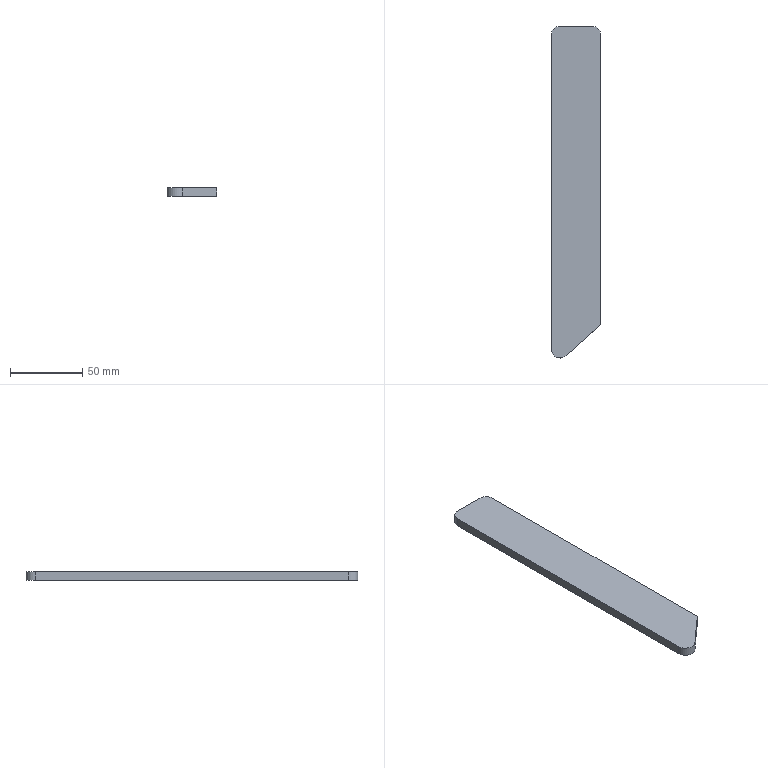Part | SolidWorks | features FlatPattern 1, SMBaseFlange 1, SheetMetal 1 | 1 solid | 9 faces | box 34.572 x 229.825 x 6 mm | volume 45739 mm3 | plane 6 | cylinder 3 | commonest cylinder face diameters 13 x3
STEP:
#1=CARTESIAN_POINT('',(34.572,168.202,0.));
#2=VERTEX_POINT('',#1);
#3=CARTESIAN_POINT('',(34.572,368.497,0.));
#4=VERTEX_POINT('',#3);
#5=CARTESIAN_POINT('',(34.572,168.202,0.));
#6=DIRECTION('',(0.,1.,0.));
#7=VECTOR('',#6,1000.);
#8=LINE('',#5,#7);
#9=EDGE_CURVE('',#2,#4,#8,.T.);
#10=ORIENTED_EDGE('',*,*,#9,.F.);
#11=CARTESIAN_POINT('',(34.572,168.202,-6.));
#12=VERTEX_POINT('',#11);
#13=CARTESIAN_POINT('',(34.572,168.202,-6.));
#14=DIRECTION('',(0.,0.,1.));
#15=VECTOR('',#14,1000.);
#16=LINE('',#13,#15);
#17=EDGE_CURVE('',#12,#2,#16,.T.);
#18=ORIENTED_EDGE('',*,*,#17,.F.);
#19=CARTESIAN_POINT('',(34.572,368.497,-6.));
#20=VERTEX_POINT('',#19);
#21=CARTESIAN_POINT('',(34.572,168.202,-6.));
#22=DIRECTION('',(0.,1.,0.));
#23=VECTOR('',#22,1000.);
#24=LINE('',#21,#23);
#25=EDGE_CURVE('',#12,#20,#24,.T.);
#26=ORIENTED_EDGE('',*,*,#25,.T.);
#27=CARTESIAN_POINT('',(34.572,368.497,-6.));
#28=DIRECTION('',(0.,0.,1.));
#29=VECTOR('',#28,1000.);
#30=LINE('',#27,#29);
#31=EDGE_CURVE('',#20,#4,#30,.T.);
#32=ORIENTED_EDGE('',*,*,#31,.T.);
#33=EDGE_LOOP('',(#10,#18,#26,#32));
#34=FACE_OUTER_BOUND('',#33,.T.);
#35=CARTESIAN_POINT('',(34.572,168.202,-6.));
#36=DIRECTION('',(1.,0.,0.));
#37=DIRECTION('',(0.,0.,-1.));
#38=AXIS2_PLACEMENT_3D('',#35,#36,#37);
#39=PLANE('',#38);
#40=ADVANCED_FACE('',(#34),#39,.T.);
#41=CARTESIAN_POINT('',(10.849,146.841,0.));
#42=VERTEX_POINT('',#41);
#43=CARTESIAN_POINT('',(10.849,146.841,0.));
#44=DIRECTION('',(0.7431,0.6691,0.));
#45=VECTOR('',#44,1000.);
#46=LINE('',#43,#45);
#47=EDGE_CURVE('',#42,#2,#46,.T.);
#48=ORIENTED_EDGE('',*,*,#47,.F.);
#49=CARTESIAN_POINT('',(10.849,146.841,-6.));
#50=VERTEX_POINT('',#49);
#51=CARTESIAN_POINT('',(10.849,146.841,-6.));
#52=DIRECTION('',(0.,0.,1.));
#53=VECTOR('',#52,1000.);
#54=LINE('',#51,#53);
#55=EDGE_CURVE('',#50,#42,#54,.T.);
#56=ORIENTED_EDGE('',*,*,#55,.F.);
#57=CARTESIAN_POINT('',(10.849,146.841,-6.));
#58=DIRECTION('',(0.7431,0.6691,0.));
#59=VECTOR('',#58,1000.);
#60=LINE('',#57,#59);
#61=EDGE_CURVE('',#50,#12,#60,.T.);
#62=ORIENTED_EDGE('',*,*,#61,.T.);
#63=ORIENTED_EDGE('',*,*,#17,.T.);
#64=EDGE_LOOP('',(#48,#56,#62,#63));
#65=FACE_OUTER_BOUND('',#64,.T.);
#66=CARTESIAN_POINT('',(10.849,146.841,-6.));
#67=DIRECTION('',(0.6691,-0.7431,0.));
#68=DIRECTION('',(0.7431,0.6691,0.));
#69=AXIS2_PLACEMENT_3D('',#66,#67,#68);
#70=PLANE('',#69);
#71=ADVANCED_FACE('',(#65),#70,.T.);
#72=CARTESIAN_POINT('',(0.,151.672,0.));
#73=VERTEX_POINT('',#72);
#74=CARTESIAN_POINT('',(6.5,151.672,0.));
#75=DIRECTION('',(0.,0.,1.));
#76=DIRECTION('',(1.,0.,0.));
#77=AXIS2_PLACEMENT_3D('',#74,#75,#76);
#78=CIRCLE('',#77,6.5);
#79=EDGE_CURVE('',#73,#42,#78,.T.);
#80=ORIENTED_EDGE('',*,*,#79,.F.);
#81=CARTESIAN_POINT('',(0.,151.672,-6.));
#82=VERTEX_POINT('',#81);
#83=CARTESIAN_POINT('',(0.,151.672,-6.));
#84=DIRECTION('',(0.,0.,1.));
#85=VECTOR('',#84,1000.);
#86=LINE('',#83,#85);
#87=EDGE_CURVE('',#82,#73,#86,.T.);
#88=ORIENTED_EDGE('',*,*,#87,.F.);
#89=CARTESIAN_POINT('',(6.5,151.672,-6.));
#90=DIRECTION('',(0.,0.,1.));
#91=DIRECTION('',(1.,0.,0.));
#92=AXIS2_PLACEMENT_3D('',#89,#90,#91);
#93=CIRCLE('',#92,6.5);
#94=EDGE_CURVE('',#82,#50,#93,.T.);
#95=ORIENTED_EDGE('',*,*,#94,.T.);
#96=ORIENTED_EDGE('',*,*,#55,.T.);
#97=EDGE_LOOP('',(#80,#88,#95,#96));
#98=FACE_OUTER_BOUND('',#97,.T.);
#99=CARTESIAN_POINT('',(6.5,151.672,-6.));
#100=DIRECTION('',(0.,0.,1.));
#101=DIRECTION('',(1.,0.,0.));
#102=AXIS2_PLACEMENT_3D('',#99,#100,#101);
#103=CYLINDRICAL_SURFACE('',#102,6.5);
#104=ADVANCED_FACE('',(#98),#103,.T.);
#105=CARTESIAN_POINT('',(0.,368.497,0.));
#106=VERTEX_POINT('',#105);
#107=CARTESIAN_POINT('',(0.,368.497,0.));
#108=DIRECTION('',(0.,-1.,0.));
#109=VECTOR('',#108,1000.);
#110=LINE('',#107,#109);
#111=EDGE_CURVE('',#106,#73,#110,.T.);
#112=ORIENTED_EDGE('',*,*,#111,.F.);
#113=CARTESIAN_POINT('',(0.,368.497,-6.));
#114=VERTEX_POINT('',#113);
#115=CARTESIAN_POINT('',(0.,368.497,-6.));
#116=DIRECTION('',(0.,0.,1.));
#117=VECTOR('',#116,1000.);
#118=LINE('',#115,#117);
#119=EDGE_CURVE('',#114,#106,#118,.T.);
#120=ORIENTED_EDGE('',*,*,#119,.F.);
#121=CARTESIAN_POINT('',(0.,368.497,-6.));
#122=DIRECTION('',(0.,-1.,0.));
#123=VECTOR('',#122,1000.);
#124=LINE('',#121,#123);
#125=EDGE_CURVE('',#114,#82,#124,.T.);
#126=ORIENTED_EDGE('',*,*,#125,.T.);
#127=ORIENTED_EDGE('',*,*,#87,.T.);
#128=EDGE_LOOP('',(#112,#120,#126,#127));
#129=FACE_OUTER_BOUND('',#128,.T.);
#130=CARTESIAN_POINT('',(0.,368.497,-6.));
#131=DIRECTION('',(-1.,0.,0.));
#132=DIRECTION('',(0.,-1.,0.));
#133=AXIS2_PLACEMENT_3D('',#130,#131,#132);
#134=PLANE('',#133);
#135=ADVANCED_FACE('',(#129),#134,.T.);
#136=CARTESIAN_POINT('',(6.5,374.997,0.));
#137=VERTEX_POINT('',#136);
#138=CARTESIAN_POINT('',(6.5,368.497,0.));
#139=DIRECTION('',(0.,0.,1.));
#140=DIRECTION('',(-1.,0.,0.));
#141=AXIS2_PLACEMENT_3D('',#138,#139,#140);
#142=CIRCLE('',#141,6.5);
#143=EDGE_CURVE('',#137,#106,#142,.T.);
#144=ORIENTED_EDGE('',*,*,#143,.F.);
#145=CARTESIAN_POINT('',(6.5,374.997,-6.));
#146=VERTEX_POINT('',#145);
#147=CARTESIAN_POINT('',(6.5,374.997,-6.));
#148=DIRECTION('',(0.,0.,1.));
#149=VECTOR('',#148,1000.);
#150=LINE('',#147,#149);
#151=EDGE_CURVE('',#146,#137,#150,.T.);
#152=ORIENTED_EDGE('',*,*,#151,.F.);
#153=CARTESIAN_POINT('',(6.5,368.497,-6.));
#154=DIRECTION('',(0.,0.,1.));
#155=DIRECTION('',(-1.,0.,0.));
#156=AXIS2_PLACEMENT_3D('',#153,#154,#155);
#157=CIRCLE('',#156,6.5);
#158=EDGE_CURVE('',#146,#114,#157,.T.);
#159=ORIENTED_EDGE('',*,*,#158,.T.);
#160=ORIENTED_EDGE('',*,*,#119,.T.);
#161=EDGE_LOOP('',(#144,#152,#159,#160));
#162=FACE_OUTER_BOUND('',#161,.T.);
#163=CARTESIAN_POINT('',(6.5,368.497,-6.));
#164=DIRECTION('',(0.,0.,1.));
#165=DIRECTION('',(1.,0.,0.));
#166=AXIS2_PLACEMENT_3D('',#163,#164,#165);
#167=CYLINDRICAL_SURFACE('',#166,6.5);
#168=ADVANCED_FACE('',(#162),#167,.T.);
#169=CARTESIAN_POINT('',(28.072,374.997,0.));
#170=VERTEX_POINT('',#169);
#171=CARTESIAN_POINT('',(28.072,374.997,0.));
#172=DIRECTION('',(-1.,0.,0.));
#173=VECTOR('',#172,1000.);
#174=LINE('',#171,#173);
#175=EDGE_CURVE('',#170,#137,#174,.T.);
#176=ORIENTED_EDGE('',*,*,#175,.F.);
#177=CARTESIAN_POINT('',(28.072,374.997,-6.));
#178=VERTEX_POINT('',#177);
#179=CARTESIAN_POINT('',(28.072,374.997,-6.));
#180=DIRECTION('',(0.,0.,1.));
#181=VECTOR('',#180,1000.);
#182=LINE('',#179,#181);
#183=EDGE_CURVE('',#178,#170,#182,.T.);
#184=ORIENTED_EDGE('',*,*,#183,.F.);
#185=CARTESIAN_POINT('',(28.072,374.997,-6.));
#186=DIRECTION('',(-1.,0.,0.));
#187=VECTOR('',#186,1000.);
#188=LINE('',#185,#187);
#189=EDGE_CURVE('',#178,#146,#188,.T.);
#190=ORIENTED_EDGE('',*,*,#189,.T.);
#191=ORIENTED_EDGE('',*,*,#151,.T.);
#192=EDGE_LOOP('',(#176,#184,#190,#191));
#193=FACE_OUTER_BOUND('',#192,.T.);
#194=CARTESIAN_POINT('',(28.072,374.997,-6.));
#195=DIRECTION('',(0.,1.,0.));
#196=DIRECTION('',(0.,0.,1.));
#197=AXIS2_PLACEMENT_3D('',#194,#195,#196);
#198=PLANE('',#197);
#199=ADVANCED_FACE('',(#193),#198,.T.);
#200=CARTESIAN_POINT('',(28.072,368.497,0.));
#201=DIRECTION('',(0.,0.,1.));
#202=DIRECTION('',(1.,0.,0.));
#203=AXIS2_PLACEMENT_3D('',#200,#201,#202);
#204=CIRCLE('',#203,6.5);
#205=EDGE_CURVE('',#4,#170,#204,.T.);
#206=ORIENTED_EDGE('',*,*,#205,.F.);
#207=ORIENTED_EDGE('',*,*,#31,.F.);
#208=CARTESIAN_POINT('',(28.072,368.497,-6.));
#209=DIRECTION('',(0.,0.,1.));
#210=DIRECTION('',(1.,0.,0.));
#211=AXIS2_PLACEMENT_3D('',#208,#209,#210);
#212=CIRCLE('',#211,6.5);
#213=EDGE_CURVE('',#20,#178,#212,.T.);
#214=ORIENTED_EDGE('',*,*,#213,.T.);
#215=ORIENTED_EDGE('',*,*,#183,.T.);
#216=EDGE_LOOP('',(#206,#207,#214,#215));
#217=FACE_OUTER_BOUND('',#216,.T.);
#218=CARTESIAN_POINT('',(28.072,368.497,-6.));
#219=DIRECTION('',(0.,0.,1.));
#220=DIRECTION('',(1.,0.,0.));
#221=AXIS2_PLACEMENT_3D('',#218,#219,#220);
#222=CYLINDRICAL_SURFACE('',#221,6.5);
#223=ADVANCED_FACE('',(#217),#222,.T.);
#224=ORIENTED_EDGE('',*,*,#25,.F.);
#225=ORIENTED_EDGE('',*,*,#61,.F.);
#226=ORIENTED_EDGE('',*,*,#94,.F.);
#227=ORIENTED_EDGE('',*,*,#125,.F.);
#228=ORIENTED_EDGE('',*,*,#158,.F.);
#229=ORIENTED_EDGE('',*,*,#189,.F.);
#230=ORIENTED_EDGE('',*,*,#213,.F.);
#231=EDGE_LOOP('',(#224,#225,#226,#227,#228,#229,#230));
#232=FACE_OUTER_BOUND('',#231,.T.);
#233=CARTESIAN_POINT('',(28.072,368.497,-6.));
#234=DIRECTION('',(0.,0.,1.));
#235=DIRECTION('',(1.,0.,0.));
#236=AXIS2_PLACEMENT_3D('',#233,#234,#235);
#237=PLANE('',#236);
#238=ADVANCED_FACE('',(#232),#237,.F.);
#239=ORIENTED_EDGE('',*,*,#9,.T.);
#240=ORIENTED_EDGE('',*,*,#205,.T.);
#241=ORIENTED_EDGE('',*,*,#175,.T.);
#242=ORIENTED_EDGE('',*,*,#143,.T.);
#243=ORIENTED_EDGE('',*,*,#111,.T.);
#244=ORIENTED_EDGE('',*,*,#79,.T.);
#245=ORIENTED_EDGE('',*,*,#47,.T.);
#246=EDGE_LOOP('',(#239,#240,#241,#242,#243,#244,#245));
#247=FACE_OUTER_BOUND('',#246,.T.);
#248=CARTESIAN_POINT('',(28.072,368.497,0.));
#249=DIRECTION('',(0.,0.,1.));
#250=DIRECTION('',(1.,0.,0.));
#251=AXIS2_PLACEMENT_3D('',#248,#249,#250);
#252=PLANE('',#251);
#253=ADVANCED_FACE('',(#247),#252,.T.);
#254=CLOSED_SHELL('',(#40,#71,#104,#135,#168,#199,#223,#238,#253));
#255=MANIFOLD_SOLID_BREP('',#254);
#256=CARTESIAN_POINT('',(0.,0.,0.));
#257=DIRECTION('',(0.,0.,1.));
#258=DIRECTION('',(1.,0.,0.));
#259=AXIS2_PLACEMENT_3D('',#256,#257,#258);
#260=(LENGTH_UNIT()NAMED_UNIT(*)SI_UNIT(.MILLI.,.METRE.));
#261=UNCERTAINTY_MEASURE_WITH_UNIT(LENGTH_MEASURE(0.00001),#260,'','');
#262=(NAMED_UNIT(*)PLANE_ANGLE_UNIT()SI_UNIT($,.RADIAN.));
#263=(NAMED_UNIT(*)SI_UNIT($,.STERADIAN.)SOLID_ANGLE_UNIT());
#264=(GEOMETRIC_REPRESENTATION_CONTEXT(3)GLOBAL_UNCERTAINTY_ASSIGNED_CONTEXT((#261))GLOBAL_UNIT_ASSIGNED_CONTEXT((#260,#262,#263))REPRESENTATION_CONTEXT('',''));
#265=ADVANCED_BREP_SHAPE_REPRESENTATION('',(#255,#259),#264);